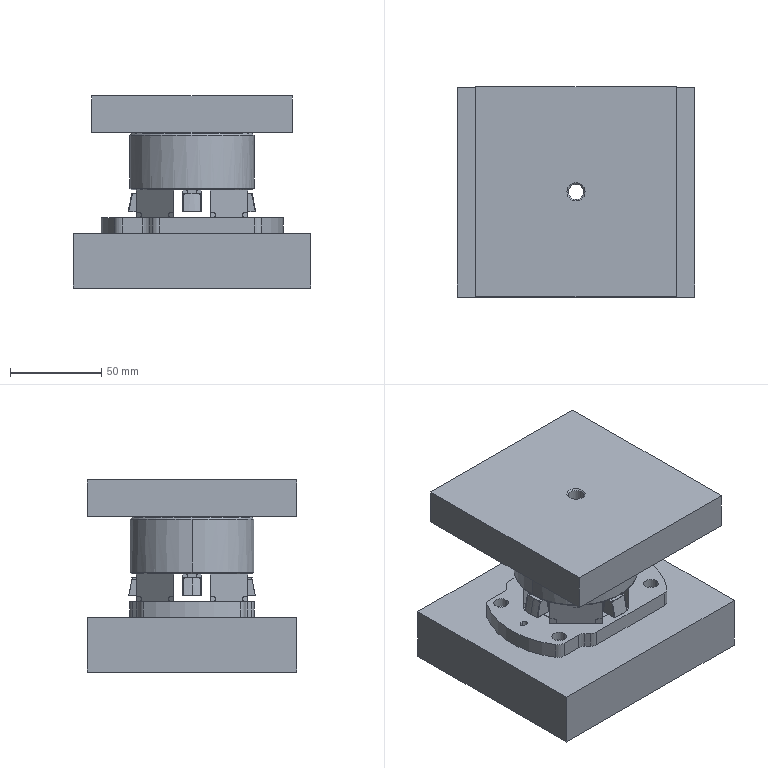NC program | NX | posted with a generic post | part box 130 x 115 x 105.2 mm
Whole program:
N10 G17 G21 G94 G90
(11 , TOOL : D50-120)
N12 T01 M6
N14 G54
N16 G17 G0 G90 X-115. Y40. B0. C0. S3000 M3
N18 G43 Z105.2 H1
N20 Z0.5
N22 G94 G1 Z0. F1000.
N24 X-90.
N26 X90.
N28 Y1.25
N30 X-90.
N32 Y-37.5
N34 X90.
N36 X115.
N38 Z0.5
N40 G0 Z105.2
N42 M5
(12 , TOOL : Φ10_CHAMFER)
N44 T02 M6
N46 G54
N48 G17 G0 G90 X-35.5 Y22.5 B0. C0. S2000 M3
N50 G43 Z105.2 H2
N52 G94 G82 G98 Z-2.2 F100. P200 R1.
N54 Y-22.5
N56 X35.5 Y22.5
N58 Y-22.5
N60 X0. Y0.
N62 G80
N64 G0 X0. Y0. Z105.2
N66 M5
(13 , TOOL : D8.6)
N68 T03 M6
N70 G54
N72 G17 G0 G90 X0. Y0. B0. C0. S1400 M3
N74 G43 Z105.2 H3
N76 G94 G82 G98 Z-35. F200. P200 R1.
N78 G80
N80 G0 X0. Y0. Z105.2
N82 M5
(14 , TOOL : ER25-D10-50)
N84 T04 M6
N86 G54
N88 G17 G0 G90 X2.995 Y-67.3 B0. C0. S5000 M3
N90 G43 Z105.2 H4
N92 G94 G1 Z-22.5 F4500.
N94 Z-23. F2500.
N96 G41 X3. Y-67. D4
N98 Y-66.
N100 G3 X0. Y-63. R3.
N102 G1 X-65.
N104 G2 X-70.5 Y-57.5 R5.5
N106 G1 Y57.5
N108 G2 X-65. Y63. R5.5
N110 G1 X65.
N112 G2 X70.5 Y57.5 R5.5
N114 G1 Y-57.5
N116 G2 X65. Y-63. R5.5
N118 G1 X0.
N120 X-0.5
N122 G3 X-3.5 Y-66. R3.
N124 G1 Y-67.
N126 G40
N128 X-3.495 Y-67.3
N130 Z-22.5
N132 G0 Z105.2
(HOLE_MILLING , TOOL : ER25-D10-50)
N134 X0. Y0.
N136 G1 Z-17.4 F4500.
N138 G3 X0.274 Y0.274 R0.274 F2500.
N140 X0. Y0.548 R0.274
N142 X-0.75 Y0. R0.787
N144 X-0.132 Y-1.093 R0.856
N146 X1.5 Y0. R1.339
N148 X0.114 Y1.86 R1.619
N150 X-2.25 Y0. R2.099
N152 X-0.108 Y-2.615 R2.375
N154 X3. Y0. R2.853
N156 X0.106 Y3.367 R3.127
N158 X-3.75 Y0. R3.606
N160 X-0.105 Y-4.119 R3.879
N162 X4.5 Y0. R4.357
N164 X0.104 Y4.87 R4.63
N166 X-5.25 Y0. R5.108
N168 X-0.104 Y-5.621 R5.381
N170 X6. Y0. R5.859
N172 X0.103 Y6.371 R6.132
N174 X-6.75 Y0. R6.609
N176 X-0.103 Y-7.122 R6.882
N178 X7.5 Y0. R7.36
N180 X0.103 Y7.872 R7.633
N182 X-8.25 Y0. R8.11
N184 X-0.103 Y-8.622 R8.383
N186 X9. Y0. R8.86
N188 X0.103 Y9.372 R9.133
N190 X-9.75 Y0. R9.611
N192 X-0.103 Y-10.123 R9.883
N194 X10.5 Y0. R10.361
N196 X0.103 Y10.873 R10.634
N198 X-11.25 Y0. R11.111
N200 X-0.103 Y-11.623 R11.384
N202 X12. Y0. R11.861
N204 X0.103 Y12.373 R12.134
N206 X-12.75 Y0. R12.611
N208 X-0.103 Y-13.123 R12.884
N210 X13.5 Y0. R13.362
N212 X0.103 Y13.873 R13.634
N214 X-14.25 Y0. R14.112
N216 X-0.103 Y-14.623 R14.384
N218 X15. Y0. R14.862
N220 X0.103 Y15.373 R15.134
N222 X-15.75 Y0. R15.612
N224 X-0.103 Y-16.123 R15.884
N226 X16.5 Y0. R16.362
N228 X0.103 Y16.874 R16.635
N230 X-17.25 Y0. R17.112
N232 X-0.103 Y-17.624 R17.385
N234 X18. Y0. R17.862
N236 X0.103 Y18.374 R18.135
N238 X-18.75 Y0. R18.612
N240 X-0.103 Y-19.124 R18.885
N242 X19.5 Y0. R19.362
N244 X0.103 Y19.874 R19.635
N246 X-20.25 Y0. R20.112
N248 X-0.103 Y-20.624 R20.385
N250 X21. Y0. R20.862
N252 X0.103 Y21.374 R21.135
N254 X-21.75 Y0. R21.612
N256 X-0.103 Y-22.124 R21.885
N258 X22.5 Y0. R22.362
N260 X0.103 Y22.874 R22.635
N262 X-23.25 Y0. R23.112
N264 X-0.103 Y-23.624 R23.385
N266 X24. Y0. R23.863
N268 X0.103 Y24.374 R24.135
N270 X-24.75 Y0. R24.613
N272 X-0.103 Y-25.124 R24.885
N274 X25.5 Y0. R25.363
N276 X0.103 Y25.874 R25.635
N278 X-26.25 Y0. R26.113
N280 X0.254 Y-26.746 R26.505
N282 X27. Y0. R26.746
N284 X27. Y0. R-27.
N286 X26.995 Y0.5 R27.
N288 X13.248 Y13.748 R13.5
N290 X0. Y0. R13.5
N292 G0 Z105.2
N294 M5
(15 , TOOL : ER25-D10-50_G)
N296 T05 M6
N298 G54
N300 G17 G0 G90 X2.995 Y-66.8 B0. C0. S5000 M3
N302 G43 Z105.2 H5
N304 G94 G1 Z-22.5 F4500.
N306 Z-23. F1000.
N308 G41 X3. Y-66.5 D5
N310 Y-65.5
N312 G3 X0. Y-62.5 R3.
N314 G1 X-65.
N316 G2 X-70. Y-57.5 R5.
N318 G1 Y57.5
N320 G2 X-65. Y62.5 R5.
N322 G1 X65.
N324 G2 X70. Y57.5 R5.
N326 G1 Y-57.5
N328 G2 X65. Y-62.5 R5.
N330 G1 X0.
N332 X-0.5
N334 G3 X-3.5 Y-65.5 R3.
N336 G1 Y-66.5
N338 G40
N340 X-3.495 Y-66.8
N342 Z-22.5
N344 G0 Z105.2
(HOLE_MILLING_COPY , TOOL : ER25-D10-50_G)
N346 X26.266 Y-0.996
N348 G1 Z-17.5 F4500.
N350 G41 X26.466 Y-1.003 F1000.
N352 G3 X27.49 Y0. R1.004
N354 X27.49 Y0. R-27.49
N356 X27.485 Y0.5 R27.49
N358 X26.443 Y1.484 R1.004
N360 G40
N362 G1 X26.244 Y1.473
N364 X26.266 Y-1.005 F4500.
N366 G41 X26.466 Y-1.013 F1000.
N368 G3 X27.5 Y0. R1.013
N370 X27.5 Y0. R-27.5
N372 X27.495 Y0.5 R27.5
N374 X26.443 Y1.494 R1.013
N376 G40
N378 G1 X26.243 Y1.483
N380 G0 Z105.2
N382 M5
(17 , TOOL : M4_D3.4)
N384 T07 M6
N386 G54
N388 G17 G0 G90 X35.5 Y22.5 B0. C0. S2000 M3
N390 G43 Z105.2 H7
N392 G94 G82 G98 Z-20. F100. P200 R1.
N394 Y-22.5
N396 X-35.5
N398 Y22.5
N400 G80
N402 G0 X-35.5 Y22.5 Z105.2
N404 M5
(PLANAR_TEXT , TOOL : Φ10_CHAMFER)
N406 T02 M6
N408 G54
N410 G17 G0 G90 X-54.593 Y48.08 B0. C0. S5000 M3
N412 G43 Z105.2 H2
N414 Z0.5
N416 G94 G1 Z-0.1 F1000.
N418 X-53.334
N420 X-52.704 Y47.922
N422 X-52.152 Y47.686
N424 X-51.759 Y47.214
N426 X-51.522 Y46.584
N428 Y46.032
N430 X-51.759 Y45.402
N432 X-52.152 Y44.93
N434 X-52.704 Y44.615
N436 X-53.097 Y44.458
N438 X-53.885 Y44.3
N440 X-54.751 Y44.221
N442 X-55.538 Y44.3
N444 X-56.326 Y44.536
N446 X-57.034 Y44.93
N448 Z4.9
N450 G0 Z105.2
N452 Y51.229
N454 Z0.5
N456 G1 Z-0.1
N458 X-56.326 Y51.623
N460 X-55.538 Y51.859
N462 X-54.751 Y51.938
N464 X-53.885 Y51.859
N466 X-53.097 Y51.702
N468 X-52.704 Y51.465
N470 X-52.152 Y51.151
N472 X-51.759 Y50.757
N474 X-51.522 Y50.127
N476 Y49.497
N478 X-51.759 Y48.946
N480 X-52.152 Y48.473
N482 X-52.704 Y48.158
N484 X-53.334 Y48.08
N486 Z4.9
N488 G0 Z105.2
N490 X-40.522 Y49.576
N492 Z0.5
N494 G1 Z-0.1
N496 X-40.759 Y48.552
N498 X-41.231 Y48.001
N500 X-41.782 Y47.686
N502 X-42.255 Y47.45
N504 X-43.042 Y47.292
N506 X-43.908
N508 X-44.696 Y47.45
N510 X-45.326 Y47.607
N512 X-45.877 Y47.922
N514 X-46.349 Y48.473
N516 X-46.664 Y49.182
N518 Y49.969
N520 X-46.428 Y50.678
N522 X-45.956 Y51.229
N524 X-45.326 Y51.544
N526 X-44.932 Y51.702
N528 X-44.145 Y51.859
N530 X-43.357 Y51.938
N532 X-42.491 Y51.78
N534 X-41.94 Y51.623
N536 X-41.31 Y51.229
N538 X-40.837 Y50.678
N540 X-40.522 Y50.048
N542 Y46.19
N544 X-40.759 Y45.481
N546 X-41.231 Y44.93
N548 X-41.861 Y44.536
N550 X-42.806 Y44.3
N552 X-43.672 Y44.221
N554 X-44.459 Y44.3
N556 X-45.247 Y44.536
N558 X-45.956 Y44.851
N560 X-46.664 Y45.402
N562 Z4.9
N564 G0 Z105.2
N566 X-29.916 Y51.938
N568 Z0.5
N570 G1 Z-0.1
N572 X-35.664
N574 Y48.473
N576 X-34.877 Y49.025
N578 X-34.089 Y49.339
N580 X-33.302 Y49.576
N582 X-32.515
N584 X-31.648 Y49.497
N586 X-30.861 Y49.261
N588 X-30.152 Y48.631
N590 X-29.68 Y47.843
N592 X-29.522 Y46.977
N594 X-29.68 Y46.032
N596 X-30.074 Y45.245
N598 X-30.782 Y44.615
N600 X-31.491 Y44.379
N602 X-31.806 Y44.3
N604 X-32.672 Y44.221
N606 X-33.459 Y44.3
N608 X-34.247 Y44.536
N610 X-34.956 Y44.851
N612 X-35.664 Y45.402
N614 Z4.9
N616 G0 Z105.2
N618 X-18.522 Y49.576
N620 Z0.5
N622 G1 Z-0.1
N624 X-18.759 Y48.552
N626 X-19.231 Y48.001
N628 X-19.782 Y47.686
N630 X-20.255 Y47.45
N632 X-21.042 Y47.292
N634 X-21.908
N636 X-22.696 Y47.45
N638 X-23.326 Y47.607
N640 X-23.877 Y47.922
N642 X-24.349 Y48.473
N644 X-24.664 Y49.182
N646 Y49.969
N648 X-24.428 Y50.678
N650 X-23.956 Y51.229
N652 X-23.326 Y51.544
N654 X-22.932 Y51.702
N656 X-22.145 Y51.859
N658 X-21.357 Y51.938
N660 X-20.491 Y51.78
N662 X-19.94 Y51.623
N664 X-19.31 Y51.229
N666 X-18.837 Y50.678
N668 X-18.522 Y50.048
N670 Y46.19
N672 X-18.759 Y45.481
N674 X-19.231 Y44.93
N676 X-19.861 Y44.536
N678 X-20.806 Y44.3
N680 X-21.672 Y44.221
N682 X-22.459 Y44.3
N684 X-23.247 Y44.536
N686 X-23.956 Y44.851
N688 X-24.664 Y45.402
N690 Z4.9
N692 G0 Z105.2
N694 X-7.522 Y50.757
N696 Z0.5
N698 G1 Z-0.1
N700 X-8.231 Y51.229
N702 X-8.94 Y51.623
N704 X-9.727 Y51.859
N706 X-10.593 Y51.938
N708 X-11.381 Y51.859
N710 X-12.326 Y51.544
N712 X-12.956 Y51.229
N714 X-13.428 Y50.678
N716 X-13.664 Y49.969
N718 Y46.111
N720 X-13.349 Y45.402
N722 X-12.877 Y44.851
N724 X-12.326 Y44.536
N726 X-11.696 Y44.379
N728 X-10.908 Y44.221
N730 X-10.042
N732 X-9.255 Y44.379
N734 X-8.861 Y44.536
N736 X-8.231 Y44.93
N738 X-7.759 Y45.481
N740 X-7.522 Y46.19
N742 Y46.899
N744 X-7.837 Y47.607
N746 X-8.31 Y48.158
N748 X-8.94 Y48.552
N750 X-9.491 Y48.71
N752 X-10.357 Y48.867
N754 X-11.145 Y48.788
N756 X-11.932 Y48.631
N758 X-12.404 Y48.473
N760 X-12.956 Y48.158
N762 X-13.428 Y47.528
N764 X-13.664 Y46.505
N766 Z4.9
N768 G0 Z105.2
N770 X3.084 Y51.938
N772 Z0.5
N774 G1 Z-0.1
N776 X-2.664
N778 Y48.473
N780 X-1.877 Y49.025
N782 X-1.089 Y49.339
N784 X-0.302 Y49.576
N786 X0.485
N788 X1.352 Y49.497
N790 X2.139 Y49.261
N792 X2.848 Y48.631
N794 X3.32 Y47.843
N796 X3.478 Y46.977
N798 X3.32 Y46.032
N800 X2.926 Y45.245
N802 X2.218 Y44.615
N804 X1.509 Y44.379
N806 X1.194 Y44.3
N808 X0.328 Y44.221
N810 X-0.459 Y44.3
N812 X-1.247 Y44.536
N814 X-1.956 Y44.851
N816 X-2.664 Y45.402
N818 Z4.9
N820 G0 Z105.2
N822 X11.643 Y51.938
N824 Z0.5
N826 G1 Z-0.1
N828 X12.43 Y51.702
N830 X12.981 Y51.308
N832 X13.926 Y50.284
N834 X14.399 Y48.788
N836 Y47.292
N838 X13.926 Y45.875
N840 X13.06 Y44.93
N842 X12.824 Y44.694
N844 X12.037 Y44.3
N846 X11.17 Y44.221
N848 X10.304 Y44.458
N850 X9.753 Y44.851
N852 X8.887 Y45.875
N854 X8.415 Y47.292
N856 Y48.788
N858 X8.887 Y50.284
N860 X9.674 Y51.229
N862 X9.989 Y51.465
N864 X10.777 Y51.859
N866 X11.643 Y51.938
N868 Z4.9
N870 G0 Z105.2
N872 X18.548 Y48.08
N874 Z0.5
N876 G1 Z-0.1
N878 X26.029
N880 Z4.9
N882 G0 Z105.2
N884 X36.635 Y49.969
N886 Z0.5
N888 G1 Z-0.1
N890 X37.107 Y50.127
N892 X37.422 Y50.048
N894 X31.438 Y49.339
N896 Z4.9
N898 G0 Z105.2
N900 X34.509 Y43.828
N902 Z0.5
N904 G1 Z-0.1
N906 X34.588 Y48.788
N908 X34.43 Y49.418
N910 Z4.9
N912 G0 Z105.2
N914 X37.501 Y44.064
N916 Z0.5
N918 G1 Z-0.1
N920 X38.21 Y44.3
N922 X38.446 Y44.143
N924 X30.572 Y43.513
N926 Z4.9
N928 G0 Z105.2
N930 X43.304 Y49.576
N932 Z0.5
N934 G1 Z-0.1
N936 X41.887 Y50.284
N938 Z4.9
N940 G0 Z105.2
N942 X44.249 Y48.631
N944 Z0.5
N946 G1 Z-0.1
N948 X41.887 Y47.45
N950 Z4.9
N952 G0 Z105.2
N954 X44.249 Y46.662
N956 Z0.5
N958 G1 Z-0.1
N960 X44.328 Y47.765
N962 Y51.308
N964 X44.407 Y51.229
N966 X44.17 Y51.544
N968 Z4.9
N970 G0 Z105.2
N972 X47.005 Y47.843
N974 Z0.5
N976 G1 Z-0.1
N978 X47.084 Y51.623
N980 X47.163 Y51.465
N982 X46.926 Y51.859
N984 Z4.9
N986 G0 Z105.2
N988 X49.525 Y49.891
N990 Z0.5
N992 G1 Z-0.1
N994 X44.958 Y49.339
N996 Z4.9
N998 G0 Z105.2
N1000 X48.895 Y48.001
N1002 Z0.5
N1004 G1 Z-0.1
N1006 X45.43 Y47.607
N1008 Z4.9
N1010 G0 Z105.2
N1012 X45.824 Y46.662
N1014 Z0.5
N1016 G1 Z-0.1
N1018 X45.43 Y47.214
N1020 Z4.9
N1022 G0 Z105.2
N1024 X48.659 Y46.269
N1026 Z0.5
N1028 G1 Z-0.1
N1030 X49.21 Y46.426
N1032 X49.446 Y46.269
N1034 X42.281 Y45.639
N1036 Z4.9
N1038 G0 Z105.2
N1040 X41.1 Y42.804
N1042 Z0.5
N1044 G1 Z-0.1
N1046 X42.123 Y43.355
N1048 X43.462 Y44.064
N1050 X44.564 Y44.851
N1052 X45.43 Y45.639
N1054 X45.667 Y45.954
N1056 Z4.9
N1058 G0 Z105.2
N1060 X46.375 Y43.434
N1062 Z0.5
N1064 G1 Z-0.1
N1066 X44.17 Y41.938
N1068 X44.328 Y42.095
N1070 X44.407 Y44.143
N1072 Y44.615
N1074 Z4.9
N1076 G0 Z105.2
N1078 X48.029 Y42.883
N1080 Z0.5
N1082 G1 Z-0.1
N1084 X48.422 Y42.568
N1086 X49.997 Y42.489
N1088 X48.501 Y42.41
N1090 X48.265 Y42.568
N1092 X47.556 Y43.276
N1094 X46.848 Y44.064
N1096 X46.218 Y44.93
N1098 X45.667 Y45.717
N1100 Z4.9
N1102 G0 Z105.2
N1104 X46.769 Y44.3
N1106 Z0.5
N1108 G1 Z-0.1
N1110 X48.029 Y45.088
N1112 X48.107 Y45.324
N1114 Z4.9
N1116 G0 Z105.2
(PLANAR_MILL_1 , TOOL : Φ10_CHAMFER)
N1118 X26.533 Y-2.995 S6500
N1120 G1 Z-1.5 F4500.
N1122 Z-2. F1000.
N1124 G41 X26.833 Y-3. D2
N1126 X28.
N1128 G3 X31. Y0. R3.
N1130 X0. Y31. R31.
N1132 X31. Y0. R-31.
N1134 X30.996 Y0.5 R31.
N1136 X27.948 Y3.451 R3.
N1138 G1 X26.781 Y3.432
N1140 G40
N1142 X26.481 Y3.422
N1144 Z-1.5
N1146 G0 Z105.2
(PLANAR_MILL_1_COPY , TOOL : Φ10_CHAMFER)
N1148 X-2.995 Y63.3
N1150 G1 Z-1.5 F4500.
N1152 Z-2. F1000.
N1154 G41 X-3. Y63.
N1156 Y62.
N1158 G3 X0. Y59. R3.
N1160 G1 X64.5
N1162 G2 X66.5 Y57. R2.
N1164 G1 Y-57.
N1166 G2 X64.5 Y-59. R2.
N1168 G1 X-64.5
N1170 G2 X-66.5 Y-57. R2.
N1172 G1 Y57.
N1174 G2 X-64.5 Y59. R2.
N1176 G1 X0.
N1178 X0.5
N1180 G3 X3.5 Y62. R3.
N1182 G1 Y63.
N1184 G40
N1186 X3.495 Y63.3
N1188 Z-1.5
N1190 G0 Z105.2
(16_COPY , TOOL : Φ10_CHAMFER)
N1192 X0. Y0. S2000
N1194 G82 G98 Z-22.5 F150. P200 R-16.5
N1196 G80
N1198 G0 X0. Y0. Z105.2
N1200 M5
N1202 M2